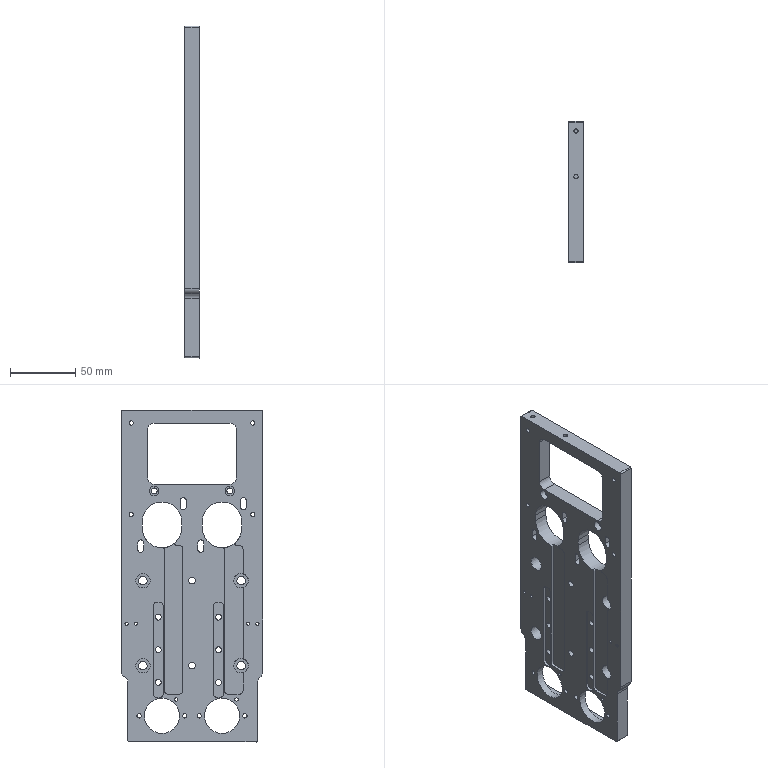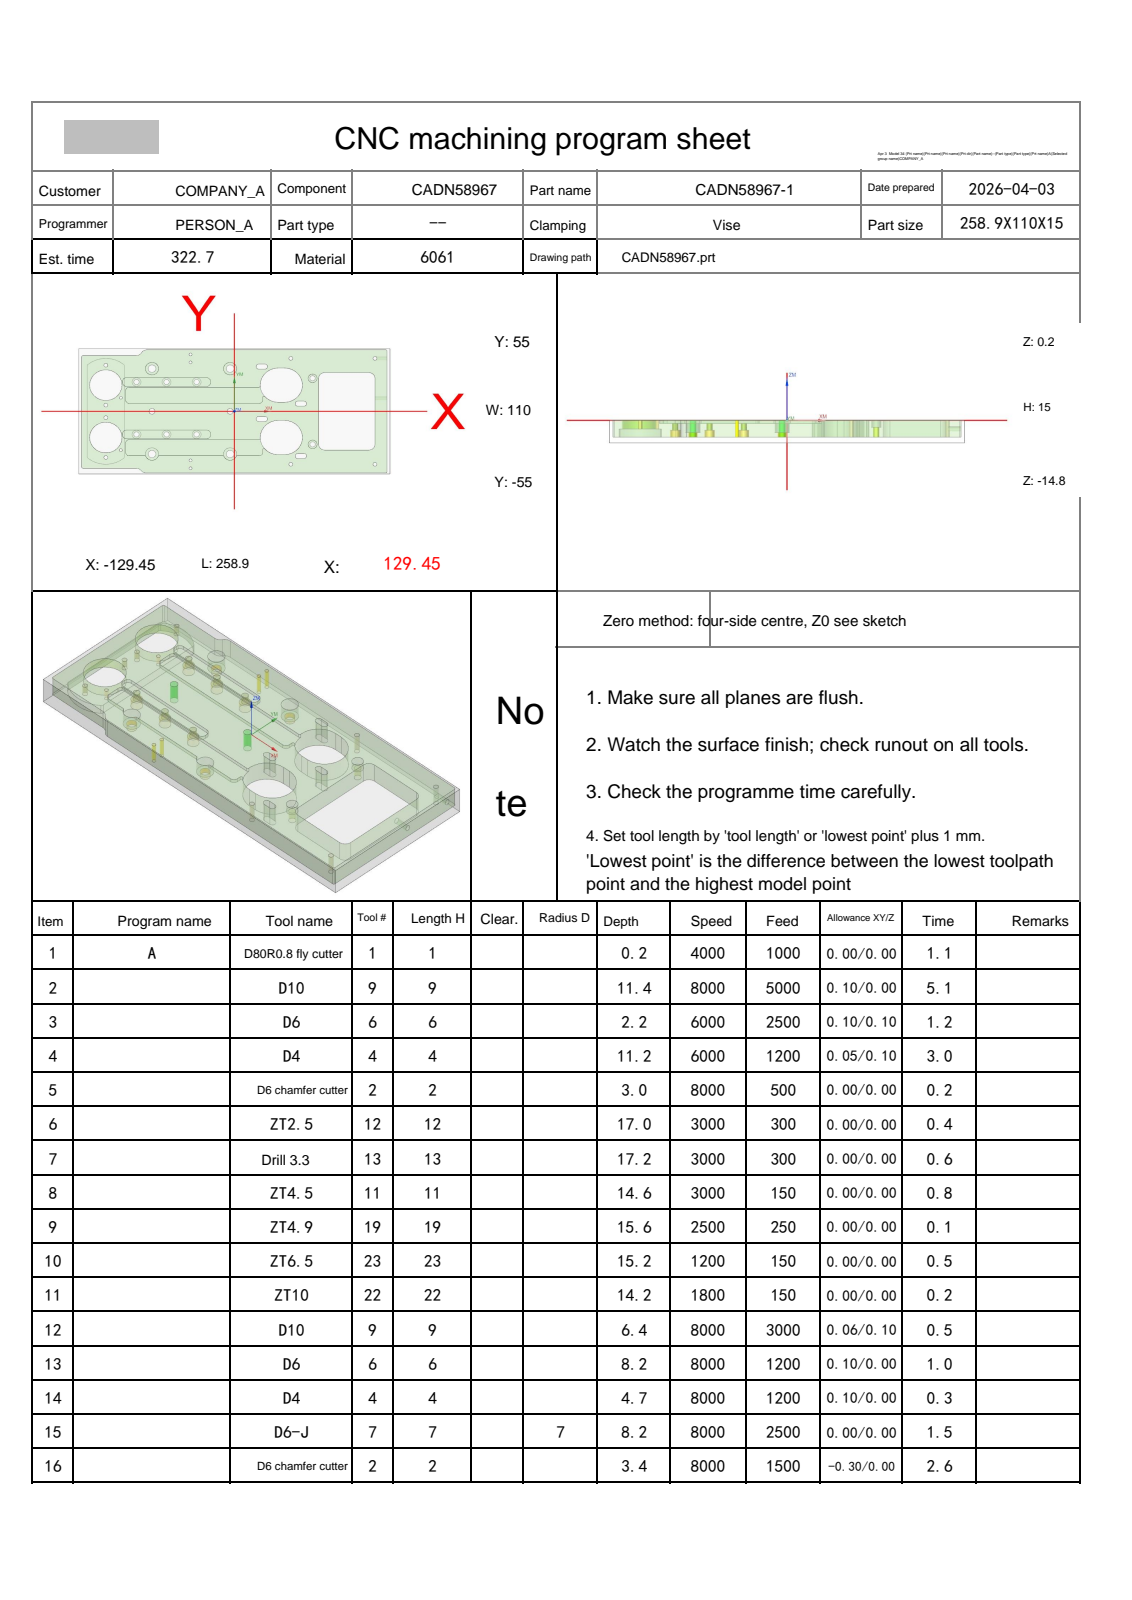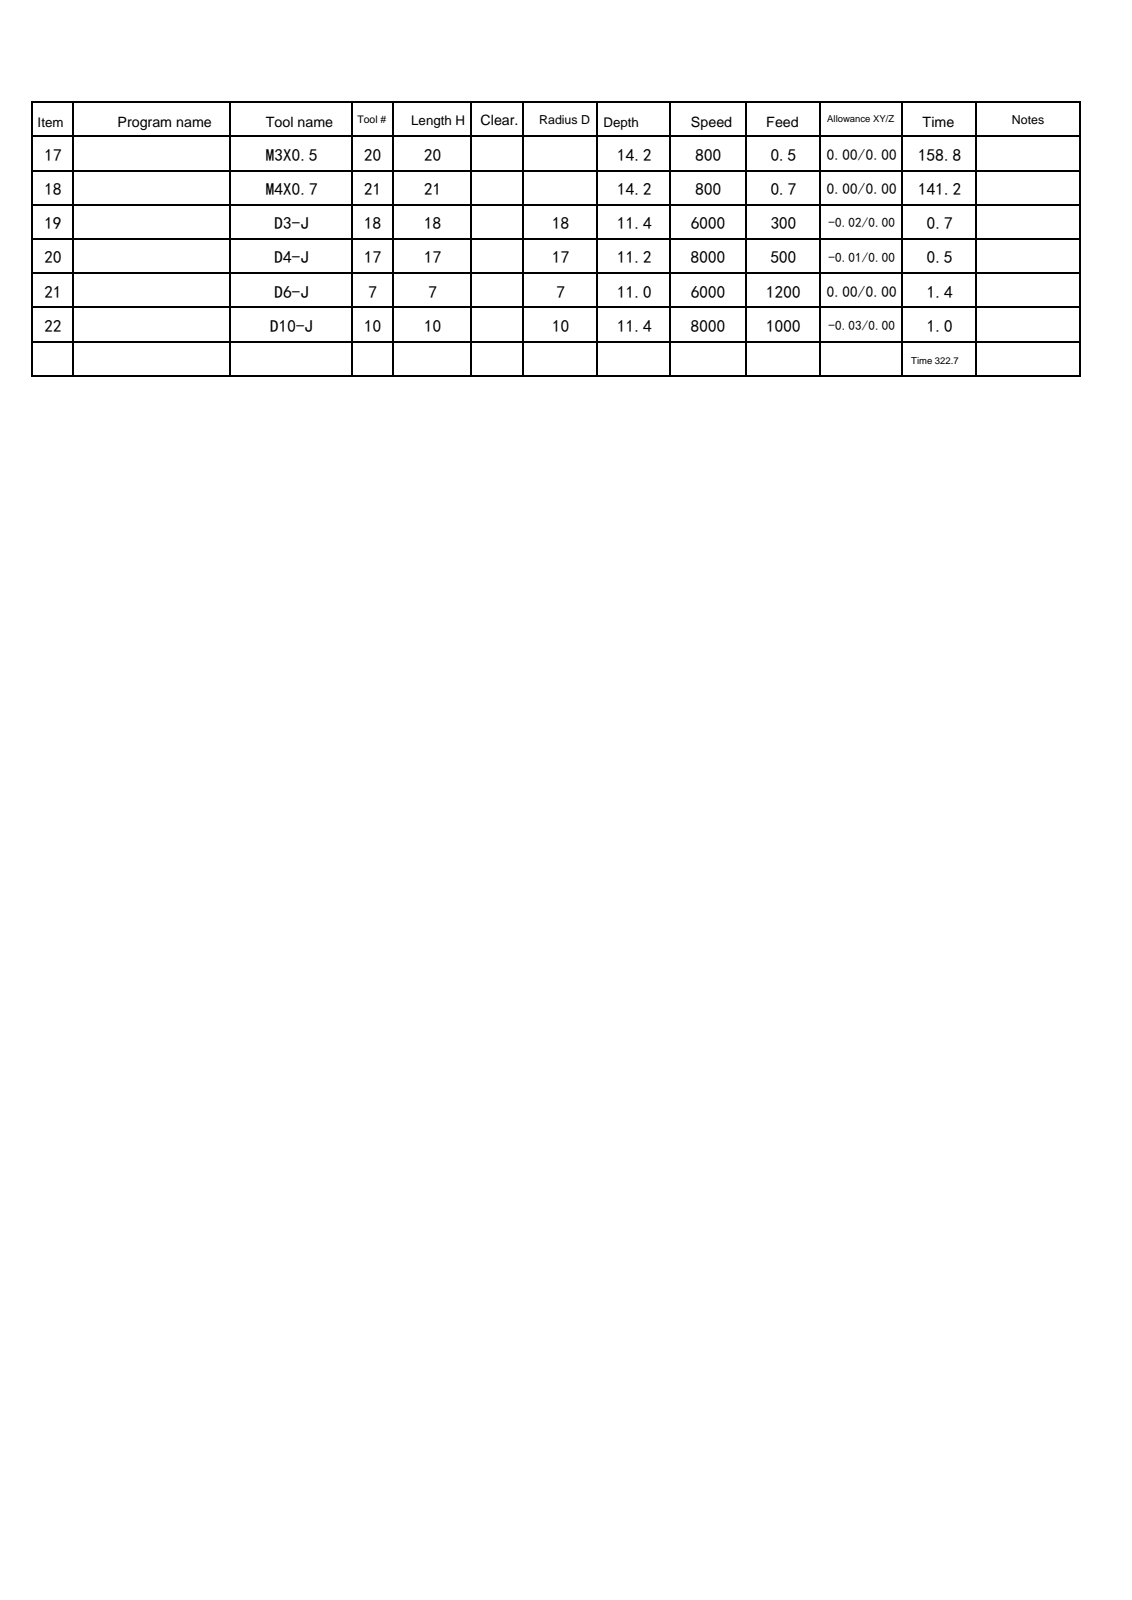NC program | NX | posted by the shop | part box 11 x 108 x 253.9 mm
Lines 4070 to 5113 of 8037:
N15 T07 M06
(D6-J  D=6. R=0. H=07 ce=0.00 di=0.00)
G00 G90 G54 X-3.55 Y-37.5 M03 S8000
G43 H07 Z20.
M08
Z0.0
G41 D07
G01 X-3.353 Y-37.468 F500.
G03 X-2.308 Y-36.242 I-.197 J1.226
X-3.55 Y-35. I-1.242 J0.0
X-3.55 Y-35. Z-5. I0.0 J-2.5
X-2.081 Y-39.523 Z-8. I0.0 J-2.5
X-1.05 Y-37.5 I-1.469 J2.023
X-3.55 Y-35. I-2.5 J0.0
X-6.05 Y-37.5 I0.0 J-2.5
X-3.55 Y-40. I2.5 J0.0
X-2.081 Y-39.523 I0.0 J2.5
X-1.569 Y-38.518 I-.73 J1.005
X-2.811 Y-37.276 I-1.242 J0.0
X-3.372 Y-37.41 I0.0 J-1.242
G01 G40 X-3.55 Y-37.5
G00 Z20.
X-68.55
Z0.0
G41 D07
G01 X-68.353 Y-37.468
G03 X-67.308 Y-36.242 I-.197 J1.226
X-68.55 Y-35. I-1.242 J0.0
X-68.55 Y-35. Z-5. I0.0 J-2.5
X-67.081 Y-39.523 Z-8. I0.0 J-2.5
X-66.05 Y-37.5 I-1.469 J2.023
X-68.55 Y-35. I-2.5 J0.0
X-71.05 Y-37.5 I0.0 J-2.5
X-68.55 Y-40. I2.5 J0.0
X-67.081 Y-39.523 I0.0 J2.5
X-66.569 Y-38.518 I-.73 J1.005
X-67.811 Y-37.276 I-1.242 J0.0
X-68.372 Y-37.41 I0.0 J-1.242
G01 G40 X-68.55 Y-37.5
G00 Z20.
Y37.5
Z0.0
G41 D07
G01 X-68.353 Y37.532
G03 X-67.308 Y38.758 I-.197 J1.226
X-68.55 Y40. I-1.242 J0.0
X-68.55 Y40. Z-5. I0.0 J-2.5
X-67.081 Y35.477 Z-8. I0.0 J-2.5
X-66.05 Y37.5 I-1.469 J2.023
X-68.55 Y40. I-2.5 J0.0
X-71.05 Y37.5 I0.0 J-2.5
X-68.55 Y35. I2.5 J0.0
X-67.081 Y35.477 I0.0 J2.5
X-66.569 Y36.482 I-.73 J1.005
X-67.811 Y37.724 I-1.242 J0.0
X-68.372 Y37.59 I0.0 J-1.242
G01 G40 X-68.55 Y37.5
G00 Z20.
X-3.55
Z0.0
G41 D07
G01 X-3.353 Y37.532
G03 X-2.308 Y38.758 I-.197 J1.226
X-3.55 Y40. I-1.242 J0.0
X-3.55 Y40. Z-5. I0.0 J-2.5
X-2.081 Y35.477 Z-8. I0.0 J-2.5
X-1.05 Y37.5 I-1.469 J2.023
X-3.55 Y40. I-2.5 J0.0
X-6.05 Y37.5 I0.0 J-2.5
X-3.55 Y35. I2.5 J0.0
X-2.081 Y35.477 I0.0 J2.5
X-1.569 Y36.482 I-.73 J1.005
X-2.811 Y37.724 I-1.242 J0.0
X-3.372 Y37.59 I0.0 J-1.242
G01 G40 X-3.55 Y37.5
G00 Z20.
G00 G90 X17.734 Y10.858 M03 S6000
Z20.
Z.615
G01 X17.735 Y10.847 Z.486 F2000.
X17.74 Y10.819 Z.37
X17.748 Y10.774 Z.265
X17.76 Y10.717 Z.171
X17.776 Y10.648 Z.087
X17.797 Y10.572 Z.014
X17.823 Y10.49 Z-.05
X17.854 Y10.406 Z-.105
X17.89 Y10.322 Z-.151
X17.933 Y10.241 Z-.19
X17.982 Y10.164 Z-.221
X18.037 Y10.096 Z-.246
X18.1 Y10.038 Z-.264
X18.17 Y9.994 Z-.276
X18.248 Y9.965 Z-.283
X18.334 Y9.955 Z-.285
X20.55 F2500.
Y12.171
X20.534 Y12.244 Z-.286
X20.487 Y12.298 Z-.288
X20.414 Y12.336 Z-.292
X20.319 Y12.358 Z-.298
X20.205 Y12.365 Z-.304
X20.077 Y12.36 Z-.312
X19.938 Y12.343 Z-.32
X19.793 Y12.315 Z-.33
X19.645 Y12.277 Z-.34
X19.498 Y12.232 Z-.35
X19.357 Y12.179 Z-.361
X19.12 Y12.068 Z-.382
X18.911 Y11.935 Z-.404
X18.73 Y11.779 Z-.426
X18.574 Y11.598 Z-.448
X18.441 Y11.39 Z-.47
X18.329 Y11.153 Z-.491
X18.276 Y11.011 Z-.503
X18.23 Y10.864 Z-.514
X18.192 Y10.715 Z-.524
X18.164 Y10.569 Z-.534
X18.146 Y10.43 Z-.542
X18.141 Y10.302 Z-.55
X18.148 Y10.187 Z-.557
X18.17 Y10.092 Z-.562
X18.207 Y10.018 Z-.567
X18.261 Y9.971 Z-.569
X18.334 Y9.955 Z-.57
X20.55
Y12.171
X20.534 Y12.244 Z-.571
X20.487 Y12.298 Z-.573
X20.414 Y12.336 Z-.577
X20.319 Y12.358 Z-.583
X20.205 Y12.365 Z-.589
X20.077 Y12.36 Z-.597
X19.938 Y12.343 Z-.605
X19.793 Y12.315 Z-.615
X19.645 Y12.277 Z-.625
X19.498 Y12.232 Z-.635
X19.357 Y12.18 Z-.646
X19.12 Y12.068 Z-.667
X18.912 Y11.935 Z-.689
X18.731 Y11.78 Z-.711
X18.575 Y11.599 Z-.733
X18.442 Y11.39 Z-.755
X18.33 Y11.153 Z-.776
X18.277 Y11.011 Z-.788
X18.231 Y10.864 Z-.799
X18.193 Y10.716 Z-.809
X18.164 Y10.57 Z-.819
X18.147 Y10.43 Z-.827
X18.141 Y10.302 Z-.835
X18.148 Y10.187 Z-.842
X18.17 Y10.092 Z-.847
X18.207 Y10.018 Z-.852
X18.261 Y9.972 Z-.854
X18.334 Y9.955 Z-.855
X20.55
Y12.171
X20.534 Y12.244 Z-.856
X20.487 Y12.298 Z-.858
X20.414 Y12.336 Z-.862
X20.319 Y12.358 Z-.868
X20.205 Y12.365 Z-.874
X20.077 Y12.36 Z-.882
X19.939 Y12.343 Z-.89
X19.793 Y12.315 Z-.9
X19.646 Y12.278 Z-.91
X19.499 Y12.232 Z-.92
X19.358 Y12.18 Z-.931
X19.121 Y12.068 Z-.952
X18.913 Y11.936 Z-.974
X18.732 Y11.78 Z-.996
X18.576 Y11.599 Z-1.018
X18.443 Y11.391 Z-1.04
X18.331 Y11.153 Z-1.061
X18.278 Y11.012 Z-1.073
X18.232 Y10.864 Z-1.084
X18.194 Y10.716 Z-1.094
X18.165 Y10.57 Z-1.104
X18.147 Y10.431 Z-1.112
X18.141 Y10.302 Z-1.12
X18.148 Y10.188 Z-1.127
X18.17 Y10.092 Z-1.132
X18.207 Y10.018 Z-1.137
X18.261 Y9.972 Z-1.139
X18.334 Y9.955 Z-1.14
X20.55
Y12.171
X20.534 Y12.244 Z-1.141
X20.487 Y12.298 Z-1.143
X20.414 Y12.336 Z-1.147
X20.319 Y12.358 Z-1.153
X20.205 Y12.365 Z-1.159
X20.077 Y12.36 Z-1.167
X19.939 Y12.343 Z-1.175
X19.794 Y12.315 Z-1.185
X19.646 Y12.278 Z-1.195
X19.5 Y12.232 Z-1.205
X19.359 Y12.18 Z-1.217
X19.122 Y12.069 Z-1.238
X18.915 Y11.936 Z-1.259
X18.734 Y11.78 Z-1.281
X18.578 Y11.599 Z-1.304
X18.445 Y11.391 Z-1.325
X18.332 Y11.154 Z-1.347
X18.279 Y11.012 Z-1.358
X18.233 Y10.865 Z-1.369
X18.195 Y10.716 Z-1.379
X18.166 Y10.57 Z-1.389
X18.148 Y10.431 Z-1.397
X18.142 Y10.302 Z-1.405
X18.149 Y10.188 Z-1.412
X18.17 Y10.092 Z-1.417
X18.207 Y10.018 Z-1.422
X18.261 Y9.972 Z-1.424
X18.334 Y9.955 Z-1.425
X20.55
Y12.171
X20.534 Y12.244 Z-1.426
X20.487 Y12.298 Z-1.428
X20.414 Y12.336 Z-1.432
X20.319 Y12.358 Z-1.438
X20.206 Y12.365 Z-1.444
X20.078 Y12.36 Z-1.452
X19.939 Y12.343 Z-1.46
X19.794 Y12.315 Z-1.47
X19.647 Y12.278 Z-1.48
X19.501 Y12.232 Z-1.491
X19.36 Y12.18 Z-1.502
X19.124 Y12.068 Z-1.523
X18.916 Y11.936 Z-1.545
X18.736 Y11.78 Z-1.567
X18.58 Y11.599 Z-1.589
X18.447 Y11.391 Z-1.611
X18.334 Y11.154 Z-1.632
X18.281 Y11.012 Z-1.643
X18.235 Y10.865 Z-1.654
X18.196 Y10.716 Z-1.664
X18.167 Y10.57 Z-1.674
X18.149 Y10.431 Z-1.683
X18.143 Y10.302 Z-1.69
X18.149 Y10.188 Z-1.697
X18.17 Y10.092 Z-1.703
X18.207 Y10.018 Z-1.707
X18.261 Y9.972 Z-1.709
X18.334 Y9.955 Z-1.71
X20.55
Y12.171
X20.534 Y12.244 Z-1.711
X20.487 Y12.298 Z-1.713
X20.414 Y12.336 Z-1.717
X20.319 Y12.358 Z-1.723
X20.206 Y12.365 Z-1.729
X20.078 Y12.36 Z-1.737
X19.94 Y12.343 Z-1.746
X19.795 Y12.315 Z-1.755
X19.648 Y12.277 Z-1.765
X19.502 Y12.232 Z-1.776
X19.361 Y12.18 Z-1.787
X19.125 Y12.068 Z-1.808
X18.918 Y11.935 Z-1.83
X18.738 Y11.78 Z-1.852
X18.582 Y11.599 Z-1.875
X18.449 Y11.391 Z-1.897
X18.336 Y11.153 Z-1.918
X18.283 Y11.011 Z-1.929
X18.236 Y10.864 Z-1.94
X18.198 Y10.716 Z-1.95
X18.169 Y10.57 Z-1.959
X18.15 Y10.431 Z-1.968
X18.143 Y10.302 Z-1.976
X18.15 Y10.188 Z-1.982
X18.171 Y10.092 Z-1.988
X18.207 Y10.018 Z-1.992
X18.261 Y9.972 Z-1.994
X18.334 Y9.955 Z-1.995
X20.55
Y12.171
X20.534 Y12.288 Z-1.985
X20.49 Y12.413 Z-1.958
X20.425 Y12.543 Z-1.914
X20.346 Y12.678 Z-1.857
X20.262 Y12.816 Z-1.788
X20.178 Y12.956 Z-1.709
X20.102 Y13.096 Z-1.623
X20.041 Y13.234 Z-1.532
X19.993 Y13.412 Z-1.405
X19.984 Y13.583 Z-1.273
X20.013 Y13.744 Z-1.14
X20.081 Y13.892 Z-1.007
X20.185 Y14.024 Z-.875
X20.326 Y14.139 Z-.748
X20.455 Y14.213 Z-.657
X20.597 Y14.279 Z-.571
X20.746 Y14.34 Z-.492
X20.895 Y14.399 Z-.423
X21.038 Y14.46 Z-.366
X21.167 Y14.525 Z-.322
X21.277 Y14.597 Z-.295
X21.36 Y14.68 Z-.285
G02 X24.55 Y16.266 I3.19 J-2.414
X25.107 Y16.227 I0.0 J-4.
G01 X25.168 Y16.221 Z-.286
X25.191 Y16.223 Z-.288
X25.179 Y16.23 Z-.292
X25.134 Y16.242 Z-.298
X25.06 Y16.256 Z-.304
X24.958 Y16.27 Z-.312
X24.832 Y16.282 Z-.321
X24.685 Y16.289 Z-.33
X24.519 Z-.34
X24.337 Y16.282 Z-.351
X24.142 Y16.263 Z-.362
X23.815 Y16.209 Z-.38
X23.472 Y16.127 Z-.399
X23.124 Y16.021 Z-.418
X22.781 Y15.893 Z-.437
X22.453 Y15.748 Z-.456
X22.149 Y15.588 Z-.475
X21.881 Y15.417 Z-.493
X21.732 Y15.305 Z-.504
X21.603 Y15.192 Z-.515
X21.493 Y15.083 Z-.525
X21.402 Y14.98 Z-.534
X21.332 Y14.886 Z-.543
X21.282 Y14.804 Z-.551
X21.254 Y14.737 Z-.557
X21.247 Y14.688 Z-.563
X21.262 Y14.66 Z-.567
X21.3 Y14.657 Z-.569
X21.36 Y14.68 Z-.57
G02 X24.55 Y16.266 I3.19 J-2.414
X25.107 Y16.227 I0.0 J-4.
G01 X25.168 Y16.221 Z-.571
X25.191 Y16.223 Z-.573
X25.178 Y16.231 Z-.577
X25.132 Y16.243 Z-.583
X25.057 Y16.257 Z-.589
X24.954 Y16.271 Z-.597
X24.828 Y16.282 Z-.605
X24.679 Y16.29 Z-.615
X24.512 Y16.291 Z-.625
X24.329 Y16.283 Z-.636
X24.133 Y16.265 Z-.647
X23.848 Y16.219 Z-.663
X23.549 Y16.152 Z-.679
X23.245 Y16.065 Z-.695
X22.942 Y15.962 Z-.712
X22.647 Y15.843 Z-.729
X22.366 Y15.711 Z-.745
X22.106 Y15.569 Z-.761
X21.874 Y15.419 Z-.777
X21.726 Y15.306 Z-.788
X21.598 Y15.194 Z-.799
X21.488 Y15.084 Z-.809
X21.399 Y14.981 Z-.819
X21.329 Y14.887 Z-.828
X21.28 Y14.804 Z-.835
X21.253 Y14.737 Z-.842
X21.246 Y14.688 Z-.847
X21.262 Y14.66 Z-.852
X21.3 Y14.657 Z-.854
X21.36 Y14.68 Z-.855
G02 X24.55 Y16.266 I3.19 J-2.414
X25.107 Y16.227 I0.0 J-4.
G01 X25.168 Y16.221 Z-.856
X25.19 Y16.223 Z-.857
X25.177 Y16.231 Z-.86
X25.131 Y16.243 Z-.864
X25.054 Y16.257 Z-.869
X24.951 Y16.271 Z-.875
X24.823 Y16.283 Z-.882
X24.674 Y16.29 Z-.89
X24.506 Y16.291 Z-.899
X24.322 Y16.284 Z-.908
X24.126 Y16.265 Z-.919
X23.839 Y16.22 Z-.934
X23.541 Y16.153 Z-.95
X23.237 Y16.067 Z-.966
X22.934 Y15.963 Z-.984
X22.639 Y15.844 Z-1.002
X22.358 Y15.712 Z-1.02
X22.099 Y15.57 Z-1.037
X21.868 Y15.42 Z-1.055
X21.721 Y15.307 Z-1.067
X21.594 Y15.195 Z-1.079
X21.485 Y15.085 Z-1.09
X21.396 Y14.982 Z-1.1
X21.327 Y14.887 Z-1.11
X21.279 Y14.805 Z-1.119
X21.251 Y14.737 Z-1.126
X21.246 Y14.688 Z-1.132
X21.261 Y14.66 Z-1.136
X21.3 Y14.657 Z-1.139
X21.36 Y14.68 Z-1.14
G02 X24.55 Y16.266 I3.19 J-2.414
X25.107 Y16.227 I0.0 J-4.
G01 X25.168 Y16.221 Z-1.141
X25.19 Y16.223 Z-1.143
X25.176 Y16.231 Z-1.146
X25.129 Y16.243 Z-1.15
X25.052 Y16.257 Z-1.156
X24.947 Y16.271 Z-1.162
X24.818 Y16.283 Z-1.169
X24.668 Y16.291 Z-1.178
X24.499 Y16.292 Z-1.187
X24.315 Y16.285 Z-1.197
X24.118 Y16.266 Z-1.207
X23.831 Y16.221 Z-1.222
X23.532 Y16.154 Z-1.238
X23.228 Y16.068 Z-1.255
X22.925 Y15.964 Z-1.272
X22.631 Y15.845 Z-1.29
X22.351 Y15.713 Z-1.307
X22.092 Y15.571 Z-1.325
X21.862 Y15.421 Z-1.342
X21.716 Y15.308 Z-1.354
X21.589 Y15.196 Z-1.365
X21.481 Y15.086 Z-1.376
X21.393 Y14.982 Z-1.386
X21.325 Y14.888 Z-1.396
X21.277 Y14.805 Z-1.404
X21.25 Y14.738 Z-1.411
X21.245 Y14.688 Z-1.417
X21.261 Y14.66 Z-1.421
X21.3 Y14.657 Z-1.424
X21.36 Y14.68 Z-1.425
G02 X24.55 Y16.266 I3.19 J-2.414
X25.107 Y16.227 I0.0 J-4.
G01 X25.168 Y16.221 Z-1.426
X25.189 Y16.223 Z-1.428
X25.175 Y16.231 Z-1.431
X25.127 Y16.243 Z-1.436
X25.049 Y16.258 Z-1.442
X24.944 Y16.272 Z-1.449
X24.814 Y16.284 Z-1.457
X24.663 Y16.291 Z-1.465
X24.493 Y16.293 Z-1.475
X24.308 Y16.285 Z-1.485
X24.11 Y16.267 Z-1.495
X23.822 Y16.222 Z-1.511
X23.523 Y16.155 Z-1.527
X23.219 Y16.069 Z-1.544
X22.917 Y15.965 Z-1.561
X22.622 Y15.846 Z-1.578
X22.343 Y15.714 Z-1.595
X22.086 Y15.572 Z-1.612
X21.856 Y15.422 Z-1.629
X21.711 Y15.309 Z-1.641
X21.585 Y15.196 Z-1.652
X21.477 Y15.087 Z-1.662
X21.39 Y14.983 Z-1.672
X21.322 Y14.888 Z-1.682
X21.275 Y14.805 Z-1.69
X21.249 Y14.738 Z-1.697
X21.244 Y14.689 Z-1.702
X21.261 Y14.66 Z-1.706
X21.299 Y14.657 Z-1.709
X21.36 Y14.68 Z-1.71
G02 X24.55 Y16.266 I3.19 J-2.414
X25.107 Y16.227 I0.0 J-4.
G01 X25.168 Y16.221 Z-1.711
X25.189 Y16.223 Z-1.713
X25.174 Y16.231 Z-1.717
X25.125 Y16.243 Z-1.722
X25.046 Y16.258 Z-1.728
X24.94 Y16.272 Z-1.735
X24.809 Y16.284 Z-1.744
X24.657 Y16.292 Z-1.753
X24.487 Y16.293 Z-1.762
X24.301 Y16.286 Z-1.773
X24.102 Y16.268 Z-1.784
X23.814 Y16.223 Z-1.799
X23.514 Y16.156 Z-1.816
X23.21 Y16.07 Z-1.832
X22.908 Y15.966 Z-1.849
X22.614 Y15.847 Z-1.866
X22.335 Y15.715 Z-1.883
X22.079 Y15.573 Z-1.9
X21.85 Y15.423 Z-1.916
X21.706 Y15.31 Z-1.927
X21.58 Y15.197 Z-1.938
X21.474 Y15.087 Z-1.949
X21.387 Y14.983 Z-1.958
X21.32 Y14.888 Z-1.967
X21.274 Y14.806 Z-1.975
X21.248 Y14.738 Z-1.982
X21.244 Y14.689 Z-1.987
X21.261 Y14.661 Z-1.992
X21.299 Y14.657 Z-1.994
X21.36 Y14.68 Z-1.995
G02 X24.55 Y16.266 I3.19 J-2.414
X25.107 Y16.227 I0.0 J-4.
G01 X25.182 Y16.235 Z-1.99
X25.243 Y16.279 Z-1.975
X25.293 Y16.353 Z-1.951
X25.331 Y16.455 Z-1.919
X25.36 Y16.579 Z-1.879
X25.378 Y16.721 Z-1.833
X25.388 Y16.877 Z-1.781
X25.391 Y17.042 Z-1.724
X25.386 Y17.213 Z-1.663
X25.375 Y17.384 Z-1.599
X25.359 Y17.552 Z-1.532
X25.316 Y17.841 Z-1.405
X25.255 Y18.108 Z-1.273
X25.173 Y18.359 Z-1.14
X25.066 Y18.598 Z-1.007
X24.932 Y18.831 Z-.875
X24.766 Y19.062 Z-.748
X24.662 Y19.189 Z-.681
X24.551 Y19.313 Z-.617
X24.435 Y19.431 Z-.556
X24.316 Y19.541 Z-.499
X24.198 Y19.638 Z-.447
X24.084 Y19.72 Z-.401
X23.975 Y19.782 Z-.361
X23.875 Y19.822 Z-.329
X23.786 Y19.836 Z-.305
X23.71 Y19.821 Z-.29
X23.652 Y19.773 Z-.285
G02 X20.47 Y18.198 I-3.182 J2.424
G01 X19.801
X19.74 Y18.194 Z-.286
X19.719 Y18.183 Z-.288
X19.734 Y18.168 Z-.292
X19.784 Y18.15 Z-.298
X19.863 Y18.132 Z-.304
X19.971 Y18.115 Z-.312
X20.103 Y18.101 Z-.321
X20.257 Y18.093 Z-.33
X20.43 Y18.092 Z-.34
X20.618 Y18.101 Z-.351
X20.819 Y18.121 Z-.362
X21.153 Y18.179 Z-.38
X21.501 Y18.266 Z-.399
X21.854 Y18.378 Z-.418
X22.201 Y18.513 Z-.437
X22.532 Y18.665 Z-.456
X22.839 Y18.832 Z-.475
X23.11 Y19.01 Z-.493
X23.261 Y19.126 Z-.504
X23.393 Y19.242 Z-.515
X23.506 Y19.355 Z-.525
X23.599 Y19.462 Z-.534
X23.671 Y19.559 Z-.543
X23.723 Y19.643 Z-.551
X23.754 Y19.712 Z-.557
X23.763 Y19.763 Z-.563
X23.749 Y19.792 Z-.567
X23.712 Y19.797 Z-.569
X23.652 Y19.773 Z-.57
G02 X20.47 Y18.198 I-3.182 J2.424
G01 X19.801
X19.74 Y18.194 Z-.571
X19.719 Y18.183 Z-.573
X19.734 Y18.168 Z-.577
X19.784 Y18.15 Z-.583
X19.863 Y18.132 Z-.589
X19.971 Y18.115 Z-.597
X20.103 Y18.101 Z-.606
X20.257 Y18.093 Z-.615
X20.43 Y18.092 Z-.625
X20.618 Y18.101 Z-.636
X20.819 Y18.121 Z-.647
X21.153 Y18.179 Z-.665
X21.501 Y18.266 Z-.684
X21.854 Y18.378 Z-.703
X22.201 Y18.513 Z-.722
X22.532 Y18.665 Z-.741
X22.839 Y18.832 Z-.76
X23.11 Y19.01 Z-.778
X23.261 Y19.126 Z-.789
X23.393 Y19.242 Z-.8
X23.506 Y19.355 Z-.81
X23.599 Y19.462 Z-.819
X23.671 Y19.559 Z-.828
X23.723 Y19.643 Z-.836
X23.754 Y19.712 Z-.842
X23.763 Y19.763 Z-.848
X23.749 Y19.792 Z-.852
X23.712 Y19.797 Z-.854
X23.652 Y19.773 Z-.855
G02 X20.47 Y18.198 I-3.182 J2.424
G01 X19.801
X19.74 Y18.194 Z-.856
X19.719 Y18.183 Z-.858
X19.734 Y18.168 Z-.862
X19.784 Y18.15 Z-.868
X19.863 Y18.132 Z-.874
X19.971 Y18.115 Z-.882
X20.103 Y18.101 Z-.891
X20.257 Y18.093 Z-.9
X20.43 Y18.092 Z-.91
X20.618 Y18.101 Z-.921
X20.819 Y18.121 Z-.932
X21.153 Y18.179 Z-.95
X21.501 Y18.266 Z-.969
X21.854 Y18.378 Z-.988
X22.201 Y18.513 Z-1.007
X22.532 Y18.665 Z-1.026
X22.839 Y18.832 Z-1.045
X23.11 Y19.01 Z-1.063
X23.261 Y19.126 Z-1.074
X23.393 Y19.242 Z-1.085
X23.506 Y19.355 Z-1.095
X23.599 Y19.462 Z-1.104
X23.671 Y19.559 Z-1.113
X23.723 Y19.643 Z-1.121
X23.754 Y19.712 Z-1.127
X23.763 Y19.763 Z-1.133
X23.749 Y19.792 Z-1.137
X23.712 Y19.797 Z-1.139
X23.652 Y19.773 Z-1.14
G02 X20.47 Y18.198 I-3.182 J2.424
G01 X19.801
X19.74 Y18.194 Z-1.141
X19.719 Y18.183 Z-1.143
X19.734 Y18.168 Z-1.147
X19.784 Y18.15 Z-1.153
X19.863 Y18.132 Z-1.159
X19.971 Y18.115 Z-1.167
X20.103 Y18.101 Z-1.176
X20.257 Y18.093 Z-1.185
X20.43 Y18.092 Z-1.195
X20.618 Y18.101 Z-1.206
X20.819 Y18.121 Z-1.217
X21.153 Y18.179 Z-1.235
X21.501 Y18.266 Z-1.254
X21.854 Y18.378 Z-1.273
X22.201 Y18.513 Z-1.292
X22.532 Y18.665 Z-1.311
X22.839 Y18.832 Z-1.33
X23.11 Y19.01 Z-1.348
X23.261 Y19.126 Z-1.359
X23.393 Y19.242 Z-1.37
X23.506 Y19.355 Z-1.38
X23.599 Y19.462 Z-1.389
X23.671 Y19.559 Z-1.398
X23.723 Y19.643 Z-1.406
X23.754 Y19.712 Z-1.412
X23.763 Y19.763 Z-1.418
X23.749 Y19.792 Z-1.422
X23.712 Y19.797 Z-1.424
X23.652 Y19.773 Z-1.425
G02 X20.47 Y18.198 I-3.182 J2.424
G01 X19.801
X19.74 Y18.194 Z-1.426
X19.719 Y18.183 Z-1.428
X19.734 Y18.168 Z-1.432
X19.784 Y18.15 Z-1.438
X19.863 Y18.132 Z-1.444
X19.971 Y18.115 Z-1.452
X20.103 Y18.101 Z-1.461
X20.257 Y18.093 Z-1.47
X20.43 Y18.092 Z-1.48
X20.618 Y18.101 Z-1.491
X20.819 Y18.121 Z-1.502
X21.153 Y18.179 Z-1.52
X21.501 Y18.266 Z-1.539
X21.854 Y18.378 Z-1.558
X22.201 Y18.513 Z-1.577
X22.532 Y18.665 Z-1.596
X22.839 Y18.832 Z-1.615
X23.11 Y19.01 Z-1.633
X23.261 Y19.126 Z-1.644
X23.393 Y19.242 Z-1.655
X23.506 Y19.355 Z-1.665
X23.599 Y19.462 Z-1.674
X23.671 Y19.559 Z-1.683
X23.723 Y19.643 Z-1.691
X23.754 Y19.712 Z-1.697
X23.763 Y19.763 Z-1.703
X23.749 Y19.792 Z-1.707
X23.712 Y19.797 Z-1.709
X23.652 Y19.773 Z-1.71
G02 X20.47 Y18.198 I-3.182 J2.424
G01 X19.801
X19.74 Y18.194 Z-1.711
X19.719 Y18.183 Z-1.713
X19.734 Y18.168 Z-1.717
X19.784 Y18.15 Z-1.723
X19.863 Y18.132 Z-1.729
X19.971 Y18.115 Z-1.737
X20.103 Y18.101 Z-1.746
X20.257 Y18.093 Z-1.755
X20.43 Y18.092 Z-1.765
X20.618 Y18.101 Z-1.776
X20.819 Y18.121 Z-1.787
X21.153 Y18.179 Z-1.805
X21.501 Y18.266 Z-1.824
X21.854 Y18.378 Z-1.843
X22.201 Y18.513 Z-1.862
X22.532 Y18.665 Z-1.881
X22.839 Y18.832 Z-1.9
X23.11 Y19.01 Z-1.918
X23.261 Y19.126 Z-1.929
X23.393 Y19.242 Z-1.94
X23.506 Y19.355 Z-1.95
X23.599 Y19.462 Z-1.959
X23.671 Y19.559 Z-1.968
X23.723 Y19.643 Z-1.976
X23.754 Y19.712 Z-1.982
X23.763 Y19.763 Z-1.988
X23.749 Y19.792 Z-1.992
X23.712 Y19.797 Z-1.994
X23.652 Y19.773 Z-1.995
G02 X20.47 Y18.198 I-3.182 J2.424
G01 X19.801
X19.715 Y18.188 Z-1.993
X19.637 Y18.159 Z-1.986
X19.567 Y18.115 Z-1.974
X19.505 Y18.057 Z-1.956
X19.449 Y17.989 Z-1.931
X19.4 Y17.913 Z-1.9
X19.358 Y17.832 Z-1.861
X19.321 Y17.748 Z-1.815
X19.29 Y17.664 Z-1.76
X19.264 Y17.582 Z-1.696
X19.243 Y17.506 Z-1.623
X19.227 Y17.438 Z-1.539
X19.215 Y17.381 Z-1.445
X19.207 Y17.336 Z-1.34
X19.202 Y17.308 Z-1.224
X19.201 Y17.298 Z-1.095
G00 Z3.
X-84.634
Z.615
G01 X-84.635 Y17.308 Z.486 F2000.
X-84.64 Y17.336 Z.37
X-84.648 Y17.381 Z.265
X-84.66 Y17.438 Z.171
X-84.676 Y17.506 Z.087
X-84.697 Y17.582 Z.014
X-84.723 Y17.664 Z-.05
X-84.754 Y17.748 Z-.105
X-84.79 Y17.832 Z-.151
X-84.833 Y17.913 Z-.19
X-84.882 Y17.989 Z-.221
X-84.937 Y18.057 Z-.246
X-85. Y18.115 Z-.264
X-85.07 Y18.159 Z-.276
X-85.148 Y18.188 Z-.283
X-85.234 Y18.198 Z-.285
X-87.45 F2500.
Y15.981
X-87.434 Y15.909 Z-.286
X-87.387 Y15.855 Z-.288
X-87.314 Y15.817 Z-.292
X-87.219 Y15.795 Z-.298
X-87.105 Y15.788 Z-.304
X-86.976 Y15.793 Z-.312
X-86.838 Y15.811 Z-.321
X-86.692 Y15.839 Z-.33
X-86.544 Y15.877 Z-.34
X-86.397 Y15.923 Z-.351
X-86.256 Y15.975 Z-.362
X-86.019 Y16.087 Z-.383
X-85.811 Y16.221 Z-.405
X-85.629 Y16.377 Z-.428
X-85.473 Y16.558 Z-.45
X-85.34 Y16.767 Z-.472
X-85.228 Y17.004 Z-.493
X-85.175 Y17.145 Z-.504
X-85.129 Y17.292 Z-.515
X-85.092 Y17.44 Z-.525
X-85.063 Y17.585 Z-.534
X-85.046 Y17.724 Z-.543
X-85.04 Y17.852 Z-.551
X-85.048 Y17.966 Z-.557
X-85.069 Y18.062 Z-.563
X-85.107 Y18.135 Z-.567
X-85.161 Y18.181 Z-.569
X-85.234 Y18.198 Z-.57
X-87.45
Y15.981
X-87.434 Y15.909 Z-.571
X-87.387 Y15.855 Z-.573
X-87.314 Y15.817 Z-.577
X-87.219 Y15.795 Z-.583
X-87.105 Y15.788 Z-.589
X-86.976 Y15.793 Z-.597
X-86.838 Y15.811 Z-.606
X-86.692 Y15.839 Z-.615
X-86.544 Y15.877 Z-.625
X-86.397 Y15.923 Z-.636
X-86.256 Y15.975 Z-.647
X-86.019 Y16.087 Z-.668
X-85.811 Y16.221 Z-.69
X-85.629 Y16.377 Z-.713
X-85.473 Y16.558 Z-.735
X-85.34 Y16.767 Z-.757
X-85.228 Y17.004 Z-.778
X-85.175 Y17.145 Z-.789
X-85.129 Y17.292 Z-.8
X-85.092 Y17.44 Z-.81
X-85.063 Y17.585 Z-.819
X-85.046 Y17.724 Z-.828
X-85.04 Y17.852 Z-.836
X-85.048 Y17.966 Z-.842
X-85.069 Y18.062 Z-.848
X-85.107 Y18.135 Z-.852
X-85.161 Y18.181 Z-.854
X-85.234 Y18.198 Z-.855
X-87.45
Y15.981
X-87.434 Y15.909 Z-.856
X-87.387 Y15.855 Z-.858
X-87.314 Y15.817 Z-.862
X-87.219 Y15.795 Z-.868
X-87.105 Y15.788 Z-.874
X-86.976 Y15.793 Z-.882
X-86.838 Y15.811 Z-.891
X-86.692 Y15.839 Z-.9
X-86.544 Y15.877 Z-.91
X-86.397 Y15.923 Z-.921
X-86.256 Y15.975 Z-.932
X-86.019 Y16.087 Z-.953
X-85.811 Y16.221 Z-.975
X-85.629 Y16.377 Z-.998
X-85.473 Y16.558 Z-1.02
X-85.34 Y16.767 Z-1.042
X-85.228 Y17.004 Z-1.063
X-85.175 Y17.145 Z-1.074
X-85.129 Y17.292 Z-1.085
X-85.092 Y17.44 Z-1.095
X-85.063 Y17.585 Z-1.104
X-85.046 Y17.724 Z-1.113
X-85.04 Y17.852 Z-1.121
X-85.048 Y17.966 Z-1.127
X-85.069 Y18.062 Z-1.133
X-85.107 Y18.135 Z-1.137
X-85.161 Y18.181 Z-1.139
X-85.234 Y18.198 Z-1.14
X-87.45
Y15.981
X-87.434 Y15.909 Z-1.141
X-87.387 Y15.855 Z-1.143
X-87.314 Y15.817 Z-1.147
X-87.219 Y15.795 Z-1.153
X-87.105 Y15.788 Z-1.159
X-86.976 Y15.793 Z-1.167
X-86.838 Y15.811 Z-1.176
X-86.692 Y15.839 Z-1.185
X-86.544 Y15.877 Z-1.195
X-86.397 Y15.923 Z-1.206
X-86.256 Y15.975 Z-1.217
X-86.019 Y16.087 Z-1.238
X-85.811 Y16.221 Z-1.26
X-85.629 Y16.377 Z-1.283
X-85.473 Y16.558 Z-1.305
X-85.34 Y16.767 Z-1.327
X-85.228 Y17.004 Z-1.348
X-85.175 Y17.145 Z-1.359
X-85.129 Y17.292 Z-1.37
X-85.092 Y17.44 Z-1.38
X-85.063 Y17.585 Z-1.389
X-85.046 Y17.724 Z-1.398
X-85.04 Y17.852 Z-1.406
X-85.048 Y17.966 Z-1.412
X-85.069 Y18.062 Z-1.418
X-85.107 Y18.135 Z-1.422
X-85.161 Y18.181 Z-1.424
X-85.234 Y18.198 Z-1.425
X-87.45
Y15.981
X-87.434 Y15.909 Z-1.426
X-87.387 Y15.855 Z-1.428
X-87.314 Y15.817 Z-1.432
X-87.219 Y15.795 Z-1.438
X-87.105 Y15.788 Z-1.444
X-86.976 Y15.793 Z-1.452
X-86.838 Y15.811 Z-1.461
X-86.692 Y15.839 Z-1.47
X-86.544 Y15.877 Z-1.48
X-86.397 Y15.923 Z-1.491
X-86.256 Y15.975 Z-1.502
X-86.019 Y16.087 Z-1.523
X-85.811 Y16.221 Z-1.545
X-85.629 Y16.377 Z-1.568
X-85.473 Y16.558 Z-1.59
X-85.34 Y16.767 Z-1.612
X-85.228 Y17.004 Z-1.633
X-85.175 Y17.145 Z-1.644
X-85.129 Y17.292 Z-1.655
X-85.092 Y17.44 Z-1.665
X-85.063 Y17.585 Z-1.674
X-85.046 Y17.724 Z-1.683
X-85.04 Y17.852 Z-1.691
X-85.048 Y17.966 Z-1.697
X-85.069 Y18.062 Z-1.703
X-85.107 Y18.135 Z-1.707
X-85.161 Y18.181 Z-1.709
X-85.234 Y18.198 Z-1.71
X-87.45
Y15.981
X-87.434 Y15.909 Z-1.711
X-87.387 Y15.855 Z-1.713
X-87.314 Y15.817 Z-1.717
X-87.219 Y15.795 Z-1.723
X-87.105 Y15.788 Z-1.729
X-86.976 Y15.793 Z-1.737
X-86.838 Y15.811 Z-1.746
X-86.692 Y15.839 Z-1.755
X-86.544 Y15.877 Z-1.765
X-86.397 Y15.923 Z-1.776
X-86.256 Y15.975 Z-1.787
X-86.019 Y16.087 Z-1.808
X-85.811 Y16.221 Z-1.83
X-85.629 Y16.377 Z-1.853
X-85.473 Y16.558 Z-1.875
X-85.34 Y16.767 Z-1.897
X-85.228 Y17.004 Z-1.918
X-85.175 Y17.145 Z-1.929
X-85.129 Y17.292 Z-1.94
X-85.092 Y17.44 Z-1.95
X-85.063 Y17.585 Z-1.959
X-85.046 Y17.724 Z-1.968
X-85.04 Y17.852 Z-1.976
X-85.048 Y17.966 Z-1.982
X-85.069 Y18.062 Z-1.988
X-85.107 Y18.135 Z-1.992
X-85.161 Y18.181 Z-1.994
X-85.234 Y18.198 Z-1.995
X-87.45
Y15.981
X-87.434 Y15.875 Z-1.987
X-87.391 Y15.757 Z-1.965
X-87.325 Y15.63 Z-1.93
X-87.243 Y15.494 Z-1.884
X-87.098 Y15.275 Z-1.794
X-86.951 Y15.054 Z-1.691
X-86.857 Y14.902 Z-1.613
X-86.775 Y14.749 Z-1.532
X-86.681 Y14.523 Z-1.405
X-86.625 Y14.299 Z-1.273
X-86.606 Y14.076 Z-1.14
X-86.625 Y13.854 Z-1.007
X-86.681 Y13.63 Z-.875
X-86.775 Y13.403 Z-.748
X-86.857 Y13.251 Z-.667
X-86.951 Y13.099 Z-.589
X-87.098 Y12.877 Z-.486
X-87.243 Y12.659 Z-.396
X-87.325 Y12.523 Z-.35
X-87.391 Y12.395 Z-.315
X-87.434 Y12.278 Z-.293
X-87.45 Y12.171 Z-.285
Y9.955
X-85.234
X-85.16 Y9.971 Z-.286
X-85.103 Y10.018 Z-.288
X-85.061 Y10.091 Z-.292
X-85.033 Y10.186 Z-.298
X-85.019 Y10.299 Z-.304
X-85.017 Y10.427 Z-.312
X-85.027 Y10.566 Z-.321
X-85.048 Y10.711 Z-.33
X-85.079 Y10.858 Z-.34
X-85.119 Y11.005 Z-.351
X-85.168 Y11.146 Z-.362
X-85.276 Y11.383 Z-.383
X-85.41 Y11.591 Z-.405
X-85.571 Y11.773 Z-.428
X-85.759 Y11.929 Z-.45
X-85.976 Y12.063 Z-.472
X-86.222 Y12.176 Z-.493
X-86.369 Y12.229 Z-.504
X-86.52 Y12.275 Z-.515
X-86.673 Y12.313 Z-.525
X-86.822 Y12.341 Z-.534
X-86.965 Y12.359 Z-.543
X-87.096 Y12.364 Z-.551
X-87.213 Y12.357 Z-.557
X-87.311 Y12.335 Z-.563
X-87.385 Y12.298 Z-.567
X-87.433 Y12.244 Z-.569
X-87.45 Y12.171 Z-.57
Y9.955
X-85.234
X-85.152 Y9.974 Z-.568
X-85.089 Y10.028 Z-.562
X-85.041 Y10.111 Z-.553
X-85.01 Y10.219 Z-.542
X-84.994 Y10.347 Z-.531
X-84.992 Y10.489 Z-.52
X-85.004 Y10.642 Z-.51
X-85.028 Y10.8 Z-.503
X-85.065 Y10.957 Z-.498
X-85.114 Y11.11 Z-.499
X-85.218 Y11.345 Z-.51
X-85.353 Y11.554 Z-.534
X-85.518 Y11.738 Z-.567
X-85.712 Y11.899 Z-.607
X-85.937 Y12.037 Z-.65
X-86.192 Y12.155 Z-.694
X-86.342 Y12.211 Z-.717
X-86.498 Y12.26 Z-.74
X-86.655 Y12.301 Z-.761
X-86.808 Y12.332 Z-.781
X-86.954 Y12.352 Z-.799
X-87.089 Y12.359 Z-.815
X-87.208 Y12.354 Z-.828
X-87.308 Y12.333 Z-.84
X-87.384 Y12.297 Z-.848
X-87.433 Y12.244 Z-.853
X-87.45 Y12.171 Z-.855
Y9.955
X-85.234
X-85.151 Y9.974 Z-.853
X-85.083 Y10.026 Z-.849
X-85.03 Y10.108 Z-.842
X-84.991 Y10.214 Z-.834
X-84.967 Y10.34 Z-.825
X-84.956 Y10.48 Z-.817
X-84.959 Y10.631 Z-.81
X-84.976 Y10.787 Z-.806
X-85.006 Y10.943 Z-.804
X-85.049 Y11.094 Z-.806
X-85.15 Y11.328 Z-.819
X-85.285 Y11.537 Z-.843
X-85.455 Y11.722 Z-.874
X-85.657 Y11.885 Z-.911
X-85.891 Y12.026 Z-.951
X-86.155 Y12.146 Z-.991
X-86.311 Y12.204 Z-1.013
X-86.472 Y12.254 Z-1.034
X-86.633 Y12.295 Z-1.053
X-86.791 Y12.327 Z-1.071
X-86.941 Y12.348 Z-1.088
X-87.08 Y12.357 Z-1.103
X-87.202 Y12.352 Z-1.116
X-87.304 Y12.333 Z-1.126
X-87.382 Y12.297 Z-1.134
X-87.432 Y12.243 Z-1.138
X-87.45 Y12.171 Z-1.14
Y9.955
X-85.234
X-85.15 Y9.973 Z-1.139
X-85.078 Y10.024 Z-1.136
X-85.019 Y10.103 Z-1.131
X-84.973 Y10.206 Z-1.126
X-84.941 Y10.329 Z-1.121
X-84.921 Y10.465 Z-1.117
X-84.916 Y10.612 Z-1.114